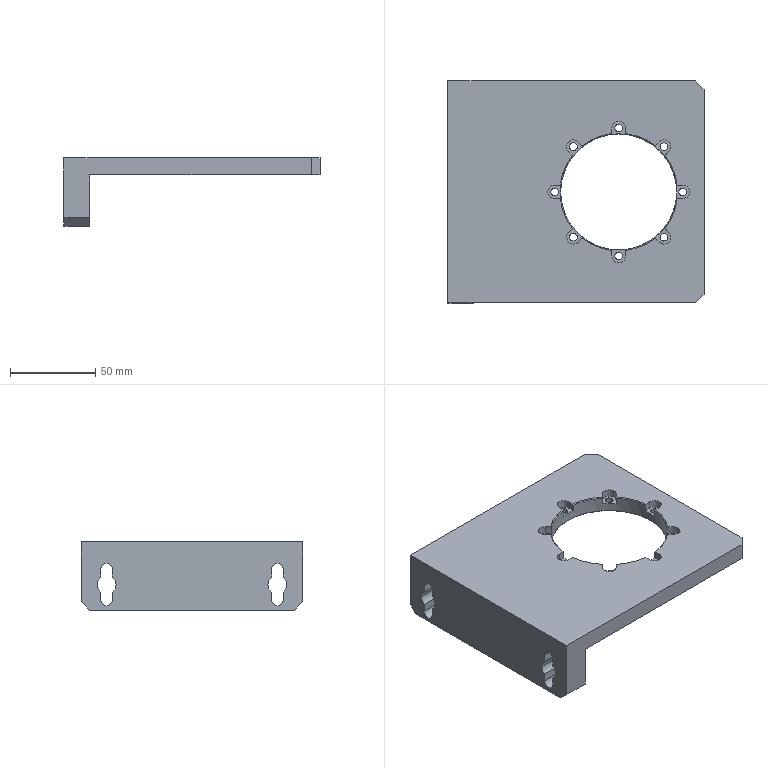NC program | NX | posted with a generic post | part box 150 x 130 x 40 mm
Lines 1 to 1320 of 2441:
N10 G17 G21 G94 G90
(FLOOR_WALL_COPY , TOOL : D80)
N12 T19 M6
N14 G54
N16 G17 G0 G90 X-123.5 Y68.497 B0. C0. S6500 M3
N18 G43 Z30. H19
N20 Z3.
N22 G94 G1 Z0. F1500.
N24 X-118.5
N26 X118.5
N28 Y15.999
N30 X-118.5
N32 Y-36.5
N34 X118.5
N36 X123.5
N38 Z3.
N40 G0 Z30.
N42 M5
(DRILLING_COPY_1 , TOOL : D6A45)
N44 T01 M6
N46 G54
N48 G17 G0 G90 X62.5 Y0. B0. C0. S5000 M3
N50 G43 Z30. H1
N52 G94 G81 G98 Z-1. F350. R3.
N54 X51.517 Y26.517
N56 X25. Y37.5
N58 X-1.517 Y26.517
N60 X-12.5 Y0.
N62 X-1.517 Y-26.517
N64 X25. Y-37.5
N66 X51.517 Y-26.517
N68 G80
N70 G0 X51.517 Y-26.517 Z30.
N72 M5
(DRILLING_COPY_COPY_COPY_2 , TOOL : 4.5ZT)
N74 T08 M6
N76 G54
N78 G17 G0 G90 X62.5 Y0. B0. C0. S2000 M3
N80 G43 Z30. H8
N82 G94 G83 G98 Z-12.852 F180. Q2. R3.
N84 X51.517 Y26.517
N86 X25. Y37.5
N88 X-1.517 Y26.517
N90 X-12.5 Y0.
N92 X-1.517 Y-26.517
N94 X25. Y-37.5
N96 X51.517 Y-26.517
N98 G80
N100 G0 X51.517 Y-26.517 Z30.
N102 M5
(ADAPTIVE_MILLING , TOOL : D10)
N104 T15 M6
N106 G54
N108 G17 G0 G90 X-90.269 Y-0.047 B0. C0. S9500 M3
N110 G43 Z30. H15
N112 Z-17.
N114 G94 G1 Z-20. F1000.
N116 X-87.817 Y-1.446 F3000.
N118 G3 X-83.547 Y-0.047 R3.035
N120 X-82.896 Y3.212 R9.612
N122 X-82.707 Y14.208 R174.736
N124 G1 X-82.705 Y22.408
N126 Y65.808
N128 X-82.703 Y65.908
N130 X-82.699 Y66.008
N132 X-82.694 Y66.108
N134 X-82.685 Y66.208
N136 G2 X-79.774 Y70.541 R6.036
N138 X-74.302 Y72.313 R13.071
N140 X-65.414 Y72.674 R78.607
N142 G1 X-63.814 Y72.681
N144 X-61.414 Y72.685
N146 X-56.914 Y72.687
N148 X75.786 Y72.688
N150 X75.886 Y72.687
N152 X75.986 Y72.683
N154 G2 X80.36 Y70.024 R5.852
N156 X82.27 Y64.605 R12.334
N158 X82.676 Y56.12 R67.698
N160 G1 X82.682 Y54.52
N162 X82.686 Y52.02
N164 X82.688 Y47.02
N166 X82.689 Y-0.98
N168 X82.696 Y-3.98
N170 X82.7 Y-6.98
N172 Y-9.98
N174 X82.696 Y-12.98
N176 X82.695 Y-13.78
N178 X82.696 Y-16.98
N180 X82.693 Y-20.08
N182 Y-20.68
N184 X82.696 Y-23.68
N186 X82.695 Y-26.68
N188 X82.693 Y-28.38
N190 X82.696 Y-31.38
N192 X82.695 Y-34.38
N194 X82.693 Y-35.98
N196 X82.696 Y-38.98
N198 X82.695 Y-41.98
N200 X82.693 Y-43.58
N202 X82.696 Y-46.58
N204 X82.695 Y-49.58
N206 X82.693 Y-51.18
N208 X82.696 Y-54.18
N210 G2 X82.665 Y-66.278 R754.805
N212 X79.782 Y-70.524 R6.056
N214 X74.315 Y-72.309 R12.987
N216 X66.028 Y-72.671 R72.365
N218 G1 X64.728 Y-72.677
N220 X62.828 Y-72.683
N222 X59.828 Y-72.686
N224 X52.328 Y-72.688
N226 X-75.772
N228 X-75.872 Y-72.687
N230 G2 X-80.233 Y-70.193 R5.761
N232 X-82.253 Y-64.714 R11.977
N234 X-82.677 Y-55.631 R69.388
N236 G1 X-82.683 Y-53.731
N238 X-82.687 Y-50.731
N240 X-82.688 Y-43.431
N242 Y-3.431
N244 X-82.686 Y-3.231
N246 X-82.684 Y-3.131
N248 G2 X-82.17 Y2.746 R196.765
N250 G3 X-81.919 Y14.44 R177.481
N252 G1 X-81.916 Y17.64
N254 X-81.914 Y25.44
N256 Y63.04
N258 X-81.913 Y63.14
N260 X-81.911 Y63.24
N262 X-81.902 Y63.44
N264 G2 X-78.052 Y69.525 R7.633
N266 X-71.898 Y71.461 R15.425
N268 X-62.412 Y71.864 R83.04
N270 G1 X-60.812 Y71.871
N272 X-58.412 Y71.875
N274 X-54.312 Y71.878
N276 X-36.512 Y71.879
N278 X73.088
N280 X73.188 Y71.878
N282 G2 X79.498 Y68.067 R7.587
N284 X81.456 Y61.921 R15.338
N286 X81.864 Y52.936 R76.536
N288 G1 X81.871 Y51.336
N290 X81.876 Y49.036
N292 X81.879 Y45.136
N294 X81.88 Y30.936
N296 Y1.736
N298 X81.889 Y-1.464
N300 X81.893 Y-4.564
N302 X81.894 Y-7.664
N304 X81.891 Y-10.764
N306 Y-11.064
N308 X81.894 Y-14.064
N310 X81.892 Y-17.064
N312 X81.89 Y-18.764
N314 X81.894 Y-21.964
N316 X81.893 Y-25.064
N318 X81.891 Y-26.964
N320 X81.894 Y-30.164
N322 Y-33.264
N324 X81.892 Y-35.564
N326 X81.894 Y-38.564
N328 X81.893 Y-41.564
N330 X81.892 Y-43.264
N332 X81.894 Y-46.264
N334 X81.893 Y-49.264
N336 X81.892 Y-50.864
N338 X81.894 Y-53.864
N340 G2 X81.859 Y-63.763 R364.257
N342 X77.841 Y-69.641 R7.736
N344 X71.558 Y-71.501 R16.073
N346 X61.469 Y-71.866 R97.349
N348 G1 X59.569 Y-71.872
N350 X56.769 Y-71.877
N352 X51.269 Y-71.879
N354 X-15.231 Y-71.88
N356 X-18.131 Y-71.887
N358 X-20.931 Y-71.89
N360 X-23.731 Y-71.889
N362 X-26.331 Y-71.885
N364 X-29.331 Y-71.887
N366 X-32.331 Y-71.884
N368 X-32.831
N370 X-35.831 Y-71.887
N372 X-38.831 Y-71.886
N374 X-40.431 Y-71.884
N376 X-43.431 Y-71.887
N378 X-46.431 Y-71.886
N380 X-48.031 Y-71.884
N382 X-51.031 Y-71.887
N384 X-54.031 Y-71.886
N386 X-55.631 Y-71.884
N388 X-58.631 Y-71.887
N390 X-61.631 Y-71.886
N392 X-63.231 Y-71.884
N394 X-66.231 Y-71.887
N396 G2 X-73.829 Y-71.845 R186.129
N398 X-79.625 Y-67.863 R7.744
N400 X-81.487 Y-61.683 R15.948
N402 X-81.863 Y-52.496 R84.129
N404 G1 X-81.87 Y-50.896
N406 X-81.875 Y-48.696
N408 X-81.878 Y-45.096
N410 X-81.88 Y-33.796
N412 X-81.879 Y-5.496
N414 X-81.876 Y-5.096
N416 G2 X-81.37 Y2.987 R183.688
N418 G3 X-81.126 Y17.983 R281.687
N420 G1 X-81.123 Y23.083
N422 X-81.122 Y60.383
N424 X-81.12 Y60.783
N426 X-81.113 Y61.083
N428 X-81.106 Y61.282
N430 G2 X-80.201 Y64.947 R9.916
N432 G3 X-79.936 Y66.425 R42.453
N434 G2 X-76.234 Y69.988 R5.268
N436 X-62.992 Y71.033 R77.349
N438 G1 X-61.792 Y71.045
N440 X-60.392 Y71.054
N442 X-58.392 Y71.062
N444 X-56.192 Y71.066
N446 X-52.192 Y71.069
N448 X-39.692 Y71.071
N450 X20.408
N452 X23.408 Y71.079
N454 X26.408 Y71.083
N456 X29.408
N458 X32.408 Y71.078
N460 X33.208 Y71.077
N462 X36.408 Y71.078
N464 X39.508 Y71.076
N466 X40.108 Y71.075
N468 X43.308 Y71.079
N470 X46.408 Y71.078
N472 X48.908 Y71.076
N474 X51.908 Y71.078
N476 X54.908 Y71.077
N478 X56.408 Y71.075
N480 X59.408 Y71.078
N482 X62.408 Y71.077
N484 X64.008 Y71.075
N486 X67.008 Y71.078
N488 G2 X72.006 Y71.008 R68.55
N490 X78.82 Y66.179 R8.85
N492 X80.698 Y59.378 R18.423
N494 X81.06 Y48.989 R104.039
N496 G1 X81.066 Y46.689
N498 X81.069 Y43.489
N500 X81.071 Y35.689
N502 Y4.389
N504 X81.081 Y1.089
N506 X81.087 Y-2.211
N508 X81.089 Y-5.511
N510 X81.087 Y-8.911
N512 X81.091 Y-12.111
N514 X81.092 Y-15.211
N516 X81.089 Y-18.311
N518 X81.093 Y-21.811
N520 X81.092 Y-24.911
N522 X81.09 Y-27.011
N524 X81.093 Y-30.211
N526 Y-33.311
N528 X81.091 Y-35.711
N530 X81.093 Y-38.711
N532 X81.092 Y-41.711
N534 X81.09 Y-43.311
N536 X81.094 Y-46.511
N538 X81.093 Y-49.611
N540 X81.091 Y-51.811
N542 X81.094 Y-54.811
N544 G2 X81.032 Y-61.909 R127.091
N546 X76.19 Y-68.822 R8.855
N548 X69.488 Y-70.683 R18.238
N550 X58.799 Y-71.06 R106.559
N552 G1 X56.499 Y-71.065
N554 X52.899 Y-71.069
N556 X44.199 Y-71.071
N558 X-12.501
N560 X-15.701 Y-71.08
N562 X-18.801 Y-71.084
N564 X-21.901 Y-71.085
N566 X-25.101 Y-71.082
N568 X-28.301 Y-71.086
N570 X-31.401
N572 X-33.901 Y-71.083
N574 X-36.901 Y-71.086
N576 X-39.901 Y-71.085
N578 X-41.501 Y-71.083
N580 X-44.501 Y-71.086
N582 X-47.501 Y-71.085
N584 X-49.101 Y-71.083
N586 X-52.301 Y-71.087
N588 X-55.401 Y-71.086
N590 X-57.901 Y-71.083
N592 X-60.901 Y-71.086
N594 X-63.901 Y-71.084
N596 X-65.101 Y-71.083
N598 X-68.101 Y-71.086
N600 G2 X-72.296 Y-70.977 R34.856
N602 X-74.971 Y-70.178 R12.895
N604 G1 X-75.067 Y-70.153
N606 X-75.165 Y-70.131
N608 X-75.187 Y-70.125
N610 X-76.234 Y-69.988
N612 X-76.331 Y-69.968
N614 X-76.425 Y-69.936
N616 G2 X-79.988 Y-66.234 R5.268
N618 X-81.039 Y-52.992 R78.181
N620 G1 X-81.049 Y-51.792
N622 X-81.057 Y-50.092
N624 X-81.064 Y-48.092
N626 X-81.068 Y-45.092
N628 X-81.071 Y-39.492
N630 Y-7.192
N632 G2 X-80.6 Y2.595 R173.692
N634 G3 X-80.335 Y19.791 R352.511
N636 G1 X-80.332 Y25.091
N638 X-80.331 Y57.691
N640 X-80.329 Y58.291
N642 X-80.324 Y58.791
N644 X-80.32 Y58.991
N646 X-80.315 Y59.191
N648 X-80.15 Y61.023
N650 G2 X-80.111 Y65.297 R63.737
N652 G1 X-79.968 Y66.331
N654 X-79.454 Y67.572
N656 X-78.637 Y68.637
N658 X-77.572 Y69.454
N660 X-76.331 Y69.968
N662 X-75.837 Y70.04
N664 X-75.099 Y70.137
N666 X-74.9 Y70.15
N668 G3 X-59.101 Y70.257 R879.606
N670 G1 X-56.601 Y70.266
N672 X-53.401 Y70.271
N674 X-52.601 Y70.272
N676 X-49.601 Y70.271
N678 X-46.601 Y70.274
N680 X-43.601 Y70.272
N682 X-40.601 Y70.273
N684 X-39.101 Y70.274
N686 X-36.101 Y70.272
N688 X-33.101 Y70.273
N690 X-31.501 Y70.274
N692 X-28.501 Y70.272
N694 X-25.501 Y70.273
N696 X-24.001 Y70.275
N698 X-21.001 Y70.272
N700 X-18.001 Y70.273
N702 X-16.401 Y70.275
N704 X-13.401 Y70.272
N706 X-10.401 Y70.273
N708 X-8.801 Y70.275
N710 X-5.801 Y70.272
N712 X-2.801 Y70.273
N714 X-1.301 Y70.275
N716 X1.699 Y70.272
N718 X4.699 Y70.273
N720 X6.299 Y70.275
N722 X9.299 Y70.272
N724 X12.299 Y70.273
N726 X13.899 Y70.274
N728 X16.899 Y70.272
N730 X19.899 Y70.273
N732 X22.899 Y70.278
N734 X24.899 Y70.283
N736 X27.899 Y70.285
N738 X28.499
N740 X31.499 Y70.282
N742 X34.499
N744 X35.399 Y70.283
N746 X38.399 Y70.278
N748 X41.399
N750 X44.399 Y70.281
N752 X47.399 Y70.279
N754 X50.399 Y70.28
N756 X51.599 Y70.282
N758 X54.599 Y70.279
N760 X57.599 Y70.28
N762 X59.199 Y70.281
N764 X62.199 Y70.279
N766 G2 X70.097 Y70.216 R155.086
N768 X77.918 Y64.879 R9.64
N770 G3 X79.399 Y62.654 R9.765
N772 G2 X80.15 Y59.9 R5.821
N774 G3 X80.255 Y49.201 R795.028
N776 G1 X80.265 Y46.901
N778 X80.271 Y43.701
N780 X80.272 Y43.401
N782 Y40.401
N784 X80.275 Y37.901
N786 X80.272 Y34.901
N788 X80.273 Y31.901
N790 X80.275 Y30.601
N792 X80.272 Y27.601
N794 X80.273 Y24.601
N796 X80.275 Y23.001
N798 X80.272 Y20.001
N800 X80.273 Y17.001
N802 X80.275 Y15.401
N804 X80.272 Y12.401
N806 X80.273 Y9.401
N808 X80.275 Y7.801
N810 X80.272 Y4.801
N812 Y3.801
N814 X80.281 Y0.601
N816 X80.286 Y-2.499
N818 X80.287 Y-5.599
N820 X80.285 Y-8.299
N822 X80.29 Y-11.499
N824 Y-14.599
N826 X80.288 Y-17.699
N828 X80.291 Y-20.899
N830 Y-23.999
N832 X80.289 Y-26.299
N834 X80.292 Y-29.499
N836 Y-32.599
N838 X80.289 Y-35.099
N840 X80.292 Y-38.099
N842 X80.291 Y-41.099
N844 X80.289 Y-42.599
N846 G2 X80.258 Y-59.698 R947.533
N848 X74.891 Y-67.919 R9.657
N850 G3 X72.654 Y-69.399 R9.648
N852 G2 X69.9 Y-70.15 R5.821
N854 G3 X59.301 Y-70.254 R763.229
N856 G1 X57.101 Y-70.263
N858 X53.901 Y-70.27
N860 X50.601 Y-70.271
N862 X48.501 Y-70.274
N864 X45.501 Y-70.272
N866 X42.501 Y-70.273
N868 X41.301 Y-70.274
N870 X38.301 Y-70.272
N872 X35.301 Y-70.273
N874 X33.701 Y-70.274
N876 X30.701 Y-70.272
N878 X27.701 Y-70.273
N880 X26.201 Y-70.274
N882 X23.201 Y-70.272
N884 X20.201 Y-70.273
N886 X18.601 Y-70.275
N888 X15.601 Y-70.272
N890 X12.601 Y-70.273
N892 X11.001 Y-70.275
N894 X8.001 Y-70.272
N896 X5.001 Y-70.273
N898 X3.501 Y-70.274
N900 X0.501 Y-70.272
N902 X-2.499 Y-70.273
N904 X-4.099 Y-70.275
N906 X-7.099 Y-70.272
N908 X-10.099 Y-70.273
N910 X-13.099 Y-70.278
N912 X-15.099 Y-70.283
N914 X-18.099 Y-70.285
N916 X-20.099 Y-70.288
N918 X-23.099 Y-70.286
N920 X-26.099 Y-70.288
N922 X-27.399 Y-70.29
N924 X-30.399 Y-70.288
N926 X-33.399 Y-70.289
N928 X-34.299 Y-70.29
N930 X-37.299 Y-70.287
N932 X-40.299 Y-70.288
N934 X-42.099 Y-70.29
N936 X-45.099 Y-70.287
N938 X-48.099 Y-70.288
N940 X-49.799 Y-70.29
N942 X-52.799 Y-70.288
N944 X-55.799 Y-70.289
N946 X-56.499
N948 X-59.399 Y-70.286
N950 G2 X-69.798 Y-70.245 R420.97
N952 G1 X-69.997 Y-70.231
N954 X-70.197 Y-70.213
N956 X-70.396 Y-70.192
N958 X-70.594 Y-70.168
N960 X-70.694 Y-70.158
N962 X-70.793 Y-70.15
N964 X-74.9
N966 X-75.099 Y-70.137
N968 X-75.198 Y-70.124
N970 G3 X-76.434 Y-70.217 R3.145
N972 G1 X-81.889 Y-71.791
N974 G2 X-85.759 Y-68.817 R3.033
N976 G1 Z-17.
N978 G0 Z30.
N980 X-82.829 Y73.315
N982 Z-17.
N984 G1 Z-20. F1000.
N986 G2 X-78.303 Y75.887 R3.033 F3000.
N988 G1 X-68.896 Y70.545
N990 G3 X-67.4 Y70.15 R3.105
N992 G1 X69.9
N994 X70.099 Y70.137
N996 G2 X73.562 Y68.702 R5.4
N998 G1 X73.712 Y68.571
N1000 X78.571 Y63.712
N1002 X79.022 Y63.15
N1004 X79.454 Y62.572
N1006 X79.968 Y61.331
N1008 X80.071 Y60.617
N1010 X80.15 Y59.9
N1012 Y-59.9
N1014 X80.137 Y-60.099
N1016 G2 X78.702 Y-63.562 R5.4
N1018 G1 X78.571 Y-63.712
N1020 X73.712 Y-68.571
N1022 X73.15 Y-69.022
N1024 X72.572 Y-69.454
N1026 X71.331 Y-69.968
N1028 X70.617 Y-70.071
N1030 X69.9 Y-70.15
N1032 X-74.9
N1034 X-75.617 Y-70.071
N1036 X-76.331 Y-69.968
N1038 X-77.572 Y-69.454
N1040 X-78.637 Y-68.637
N1042 X-79.454 Y-67.572
N1044 X-79.968 Y-66.331
N1046 X-80.053 Y-65.738
N1048 X-80.137 Y-65.099
N1050 X-80.15 Y-64.9
N1052 G3 X-80.254 Y-50.001 R826.107
N1054 G1 X-80.264 Y-47.601
N1056 X-80.271 Y-44.401
N1058 Y-44.001
N1060 X-80.272 Y-41.001
N1062 X-80.274 Y-38.501
N1064 X-80.272 Y-35.501
N1066 X-80.274 Y-32.501
N1068 X-80.275 Y-31.301
N1070 X-80.272 Y-28.301
N1072 X-80.273 Y-25.301
N1074 X-80.275 Y-23.701
N1076 X-80.272 Y-20.701
N1078 X-80.273 Y-17.701
N1080 X-80.275 Y-16.101
N1082 X-80.272 Y-13.101
N1084 G2 X-80.15 Y-3.703 R204.302
N1086 G1 Y61.097
N1088 G3 X-81.032 Y63.343 R3.335
N1090 X-83.137 Y64.382 Z-19.9 R3.335
N1092 X-86.75 Y61.097 R3.305
N1094 G1 Y-57.6
N1096 G3 X-82.982 Y-60.867 R3.305
N1098 X-80.928 Y-59.729 Z-20. R3.335
N1100 X-80.15 Y-57.6 R3.336
N1102 G1 Y-3.7
N1104 G3 X-83.078 Y-0.672 R3.036
N1106 G1 X-86.343 Y-0.562
N1108 Z-17.
N1110 G0 Z30.
N1112 X-90.271 Y-0.049
N1114 Z-37.
N1116 G1 Z-40. F1000.
N1118 X-87.819 Y-1.448 F3000.
N1120 G3 X-83.549 Y-0.049 R3.035
N1122 X-82.898 Y3.21 R9.612
N1124 X-82.709 Y14.207 R174.736
N1126 G1 X-82.707 Y22.407
N1128 Y65.807
N1130 X-82.705 Y65.907
N1132 X-82.701 Y66.007
N1134 X-82.695 Y66.106
N1136 X-82.687 Y66.206
N1138 G2 X-79.778 Y70.541 R6.037
N1140 X-74.307 Y72.314 R13.032
N1142 X-65.419 Y72.676 R78.45
N1144 G1 X-63.919 Y72.682
N1146 X-61.619 Y72.687
N1148 X-57.419 Y72.689
N1150 X-27.519 Y72.69
N1152 X75.781
N1154 X75.881 Y72.689
N1156 G2 X80.24 Y70.191 R5.757
N1158 X82.27 Y64.611 R12.073
N1160 X82.667 Y56.727 R62.897
N1162 G1 X82.676 Y55.527
N1164 X82.682 Y53.927
N1166 X82.687 Y51.627
N1168 X82.689 Y47.527
N1170 X82.69 Y14.427
N1172 X82.691 Y-7.273
N1174 X82.698 Y-10.273
N1176 X82.702 Y-13.273
N1178 Y-16.273
N1180 X82.698 Y-19.273
N1182 X82.697 Y-20.073
N1184 X82.698 Y-23.273
N1186 X82.695 Y-26.373
N1188 Y-26.973
N1190 X82.698 Y-29.973
N1192 X82.697 Y-32.973
N1194 X82.695 Y-34.673
N1196 X82.698 Y-37.673
N1198 X82.697 Y-40.673
N1200 X82.695 Y-42.273
N1202 X82.698 Y-45.273
N1204 X82.697 Y-48.273
N1206 X82.695 Y-49.873
N1208 X82.698 Y-52.873
N1210 X82.697 Y-55.873
N1212 X82.695 Y-57.473
N1214 X82.698 Y-60.473
N1216 G2 X82.658 Y-66.371 R131.179
N1218 X79.624 Y-70.628 R6.152
N1220 X74.129 Y-72.335 R13.448
N1222 X65.04 Y-72.682 R83.457
N1224 G1 X62.74 Y-72.687
N1226 X58.44 Y-72.689
N1228 X8.74 Y-72.69
N1230 X-75.86 Y-72.689
N1232 X-75.96 Y-72.686
N1234 X-76.06 Y-72.681
N1236 G2 X-80.459 Y-69.881 R5.939
N1238 X-82.295 Y-64.433 R12.732
N1240 X-82.678 Y-55.147 R77.923
N1242 G1 X-82.684 Y-53.447
N1244 X-82.688 Y-50.847
N1246 X-82.69 Y-45.447
N1248 Y-3.347
N1250 X-82.686 Y-3.147
N1252 X-82.681 Y-2.947
N1254 G2 X-82.147 Y3.129 R700.412
N1256 G3 X-81.918 Y17.225 R247.329
N1258 G1 X-81.916 Y23.825
N1260 Y63.025
N1262 X-81.915 Y63.125
N1264 X-81.913 Y63.225
N1266 X-81.905 Y63.425
N1268 X-81.892 Y63.624
N1270 G2 X-77.984 Y69.571 R7.687
N1272 X-71.719 Y71.486 R15.754
N1274 X-61.732 Y71.868 R93.067
N1276 G1 X-59.932 Y71.874
N1278 X-57.432 Y71.878
N1280 X-52.632 Y71.881
N1282 X60.968
N1284 X73.068
N1286 X73.168 Y71.88
N1288 G2 X79.489 Y68.087 R7.588
N1290 X81.478 Y61.745 R15.429
N1292 X81.864 Y52.358 R85.367
N1294 G1 X81.871 Y50.858
N1296 X81.876 Y48.758
N1298 X81.88 Y45.458
N1300 X81.881 Y37.358
N1302 X81.882 Y-4.542
N1304 X81.891 Y-7.742
N1306 X81.895 Y-10.842
N1308 X81.896 Y-13.942
N1310 X81.893 Y-17.042
N1312 Y-17.342
N1314 X81.896 Y-20.342
N1316 X81.894 Y-23.342
N1318 X81.892 Y-25.042
N1320 X81.895 Y-28.242
N1322 X81.894 Y-31.342
N1324 X81.893 Y-33.242
N1326 X81.896 Y-36.442
N1328 Y-39.542
N1330 X81.893 Y-41.842
N1332 X81.896 Y-44.842
N1334 X81.895 Y-47.842
N1336 X81.893 Y-49.542
N1338 X81.896 Y-52.542
N1340 X81.895 Y-55.542
N1342 X81.893 Y-57.142
N1344 X81.896 Y-60.142
N1346 G2 X81.815 Y-64.138 R36.087
N1348 X77.602 Y-69.779 R7.882
N1350 X71.185 Y-71.546 R17.008
N1352 X61.695 Y-71.868 R100.448
N1354 G1 X59.895 Y-71.875
N1356 X57.295 Y-71.879
N1358 X52.095 Y-71.881
N1360 X-73.105
N1362 X-73.205 Y-71.879
N1364 X-73.405 Y-71.873
N1366 G2 X-79.508 Y-68.052 R7.626
N1368 X-81.459 Y-61.904 R15.357
N1370 X-81.862 Y-52.618 R81.436
N1372 G1 X-81.87 Y-51.218
N1374 X-81.875 Y-49.418
N1376 X-81.879 Y-46.618
N1378 X-81.881 Y-40.818
N1380 Y-5.518
N1382 X-81.88 Y-5.318
N1384 G2 X-81.389 Y2.765 R158.22
N1386 G3 X-81.129 Y17.161 R254.609
N1388 G1 X-81.126 Y21.361
N1390 X-81.125 Y34.261
N1392 X-81.124 Y60.361
N1394 X-81.122 Y60.761
N1396 X-81.116 Y61.06
N1398 X-81.108 Y61.26
N1400 G2 X-80.18 Y65.021 R10.687
N1402 G1 X-80.154 Y65.118
N1404 X-80.13 Y65.215
N1406 X-80.109 Y65.313
N1408 X-79.988 Y66.234
N1410 X-79.968 Y66.331
N1412 X-79.936 Y66.425
N1414 G2 X-76.234 Y69.988 R5.268
N1416 X-62.892 Y71.035 R77.561
N1418 G1 X-61.692 Y71.046
N1420 X-60.292 Y71.055
N1422 X-58.392 Y71.063
N1424 X-56.192 Y71.068
N1426 X-52.392 Y71.071
N1428 X-42.192 Y71.072
N1430 X-2.992 Y71.073
N1432 X0.008 Y71.081
N1434 X3.008 Y71.085
N1436 X6.008 Y71.084
N1438 X9.008 Y71.08
N1440 X9.808 Y71.079
N1442 X13.008 Y71.08
N1444 X16.108 Y71.078
N1446 X16.708 Y71.077
N1448 X19.908 Y71.081
N1450 X23.008 Y71.08
N1452 X25.508 Y71.077
N1454 X28.708 Y71.081
N1456 X31.808 Y71.08
N1458 X34.008 Y71.077
N1460 X37.008 Y71.08
N1462 X40.008 Y71.079
N1464 X41.408 Y71.077
N1466 X44.408 Y71.08
N1468 X47.408 Y71.079
N1470 X49.008 Y71.077
N1472 X52.008 Y71.08
N1474 X55.008 Y71.079
N1476 X56.608 Y71.077
N1478 X59.808 Y71.081
N1480 G2 X71.707 Y71.039 R440.492
N1482 X78.724 Y66.358 R8.791
N1484 X80.684 Y59.481 R17.918
N1486 X81.06 Y48.492 R113.184
N1488 G1 X81.066 Y46.392
N1490 X81.07 Y43.492
N1492 X81.073 Y37.592
N1494 Y-1.808
N1496 X81.082 Y-5.008
N1498 X81.087 Y-8.108
N1500 X81.088 Y-11.908
N1502 X81.087 Y-15.908
N1504 X81.095 Y-19.108
N1506 X81.098 Y-22.208
N1508 Y-25.308
N1510 X81.093 Y-28.408
N1512 X81.092 Y-29.408
N1514 X81.093 Y-32.408
N1516 X81.091 Y-34.508
N1518 X81.096 Y-37.508
N1520 Y-40.508
N1522 X81.093 Y-43.408
N1524 X81.096 Y-46.608
N1526 X81.095 Y-49.708
N1528 X81.092 Y-51.908
N1530 X81.095 Y-54.908
N1532 X81.094 Y-57.908
N1534 X81.092 Y-59.108
N1536 G2 X80.835 Y-63.088 R16.768
N1538 X75.843 Y-69.006 R9.072
N1540 X68.999 Y-70.74 R19.471
N1542 X58.107 Y-71.062 R129.678
N1544 G1 X55.907 Y-71.067
N1546 X52.507 Y-71.071
N1548 X44.007 Y-71.072
N1550 X-70.693
N1552 X-70.993 Y-71.069
N1554 X-71.093 Y-71.066
N1556 G2 X-74.868 Y-70.203 R9.973
N1558 G1 X-74.964 Y-70.176
N1560 X-75.061 Y-70.152
N1562 X-75.168 Y-70.128
N1564 X-76.234 Y-69.988
N1566 X-76.331 Y-69.968
N1568 X-76.425 Y-69.936
N1570 G2 X-79.988 Y-66.234 R5.268
N1572 X-81.049 Y-52.292 R81.817
N1574 G1 X-81.057 Y-50.792
N1576 X-81.065 Y-48.592
N1578 X-81.069 Y-45.792
N1580 X-81.072 Y-40.892
N1582 X-81.073 Y-11.392
N1584 X-81.072 Y-7.092
N1586 G2 X-80.606 Y2.595 R173.405
N1588 G3 X-80.337 Y19.091 R338.312
N1590 G1 X-80.334 Y23.591
N1592 X-80.333 Y37.691
N1594 Y57.591
N1596 X-80.33 Y58.391
N1598 X-80.326 Y58.791
N1600 X-80.319 Y59.091
N1602 G2 X-80.15 Y61.082 R56.218
N1604 G1 Y64.9
N1606 X-80.137 Y65.099
N1608 X-80.098 Y65.396
N1610 X-79.968 Y66.331
N1612 X-79.454 Y67.572
N1614 X-78.637 Y68.637
N1616 X-77.572 Y69.454
N1618 X-76.331 Y69.968
N1620 X-75.837 Y70.04
N1622 X-75.099 Y70.137
N1624 X-74.9 Y70.15
N1626 G3 X-59.001 Y70.258 R888.706
N1628 G1 X-56.501 Y70.267
N1630 X-53.501 Y70.272
N1632 X-52.901 Y70.273
N1634 X-49.901
N1636 X-47.101 Y70.276
N1638 X-44.101 Y70.274
N1640 X-41.101 Y70.275
N1642 X-39.801 Y70.276
N1644 X-36.801 Y70.274
N1646 X-33.801 Y70.275
N1648 X-32.201 Y70.276
N1650 X-29.201 Y70.274
N1652 X-26.201 Y70.275
N1654 X-24.601 Y70.276
N1656 X-21.601 Y70.274
N1658 X-18.601 Y70.275
N1660 X-17.101 Y70.276
N1662 X-14.101 Y70.273
N1664 X-11.101 Y70.275
N1666 X-9.501 Y70.276
N1668 X-6.501 Y70.274
N1670 X-3.501 Y70.275
N1672 X-0.501 Y70.28
N1674 X1.499 Y70.285
N1676 X4.699 Y70.286
N1678 X5.499 Y70.287
N1680 X8.699 Y70.282
N1682 X11.799
N1684 X13.699 Y70.283
N1686 X16.699 Y70.278
N1688 X19.699
N1690 X22.699 Y70.281
N1692 X25.699 Y70.278
N1694 X28.699 Y70.28
N1696 X30.399 Y70.282
N1698 X33.399 Y70.28
N1700 X36.399 Y70.281
N1702 X37.599 Y70.283
N1704 X40.599 Y70.28
N1706 X43.599 Y70.281
N1708 X45.199 Y70.282
N1710 X48.199 Y70.28
N1712 X51.199 Y70.281
N1714 X52.699 Y70.282
N1716 X55.699 Y70.28
N1718 X58.699 Y70.281
N1720 X60.699 Y70.283
N1722 X63.899 Y70.28
N1724 G2 X70.197 Y70.208 R96.937
N1726 X77.965 Y64.794 R9.65
N1728 G3 X79.399 Y62.654 R9.527
N1730 G2 X80.15 Y59.9 R5.821
N1732 G3 X80.257 Y48.301 R824.167
N1734 G1 X80.267 Y46.001
N1736 X80.273 Y42.801
N1738 Y42.301
N1740 X80.274 Y39.301
N1742 X80.276 Y36.801
N1744 X80.274 Y33.801
N1746 X80.275 Y30.801
N1748 X80.277 Y29.501
N1750 X80.274 Y26.501
N1752 X80.275 Y23.501
N1754 X80.277 Y21.901
N1756 X80.274 Y18.901
N1758 X80.275 Y15.901
N1760 X80.277 Y14.301
N1762 X80.274 Y11.301
N1764 X80.275 Y8.301
N1766 X80.277 Y6.801
N1768 X80.274 Y3.801
N1770 X80.275 Y0.801
N1772 X80.28 Y-2.199
N1774 X80.285 Y-4.199
N1776 X80.287 Y-7.199
N1778 X80.29 Y-9.399
N1780 X80.289 Y-12.399
N1782 X80.291 Y-15.399
N1784 X80.298 Y-18.399
N1786 Y-18.699
N1788 X80.299 Y-21.699
N1790 X80.301 Y-23.499
N1792 X80.298 Y-26.499
N1794 X80.299 Y-29.299
N1796 X80.294 Y-32.199
N1798 X80.293 Y-34.999
N1800 X80.297 Y-37.799
N1802 X80.298 Y-38.699
N1804 X80.297 Y-41.699
N1806 X80.299 Y-44.699
N1808 X80.3 Y-45.399
N1810 X80.297 Y-48.399
N1812 X80.298 Y-51.399
N1814 X80.299 Y-52.499
N1816 X80.296 Y-55.499
N1818 Y-58.199
N1820 X80.295 Y-58.499
N1822 X80.291 Y-58.899
N1824 X80.284 Y-59.199
N1826 X80.272 Y-59.499
N1828 G2 X74.897 Y-67.92 R9.669
N1830 G3 X72.654 Y-69.399 R9.583
N1832 G2 X69.9 Y-70.15 R5.821
N1834 G3 X58.501 Y-70.257 R812.566
N1836 G1 X56.101 Y-70.266
N1838 X53.101 Y-70.272
N1840 X52.701 Y-70.273
N1842 X49.701
N1844 X47.301 Y-70.276
N1846 X44.301 Y-70.273
N1848 X41.301 Y-70.275
N1850 X39.901 Y-70.276
N1852 X36.901 Y-70.274
N1854 X33.901 Y-70.275
N1856 X32.301 Y-70.276
N1858 X29.301 Y-70.274
N1860 X26.301 Y-70.275
N1862 X24.701 Y-70.276
N1864 X21.701 Y-70.273
N1866 X18.701 Y-70.275
N1868 X17.101 Y-70.276
N1870 X14.101 Y-70.274
N1872 X11.101 Y-70.275
N1874 X9.501 Y-70.276
N1876 X6.501 Y-70.274
N1878 X3.501 Y-70.275
N1880 X2.001 Y-70.276
N1882 X-0.999 Y-70.273
N1884 X-3.999 Y-70.275
N1886 X-5.599 Y-70.276
N1888 X-8.599 Y-70.274
N1890 X-11.599 Y-70.275
N1892 X-13.099 Y-70.276
N1894 X-16.099 Y-70.274
N1896 X-19.099 Y-70.275
N1898 X-20.699 Y-70.276
N1900 X-23.699 Y-70.274
N1902 X-26.699 Y-70.275
N1904 X-28.299 Y-70.276
N1906 X-31.299 Y-70.274
N1908 X-34.299 Y-70.275
N1910 X-35.999 Y-70.276
N1912 X-38.999 Y-70.274
N1914 X-41.999 Y-70.275
N1916 X-43.599 Y-70.276
N1918 X-46.599 Y-70.274
N1920 X-49.599 Y-70.275
N1922 X-51.199 Y-70.276
N1924 X-54.199 Y-70.274
N1926 G2 X-69.698 Y-70.241 R869.795
N1928 G1 X-69.898 Y-70.228
N1930 X-70.097 Y-70.212
N1932 X-70.296 Y-70.192
N1934 X-70.495 Y-70.17
N1936 X-70.594 Y-70.159
N1938 X-70.699 Y-70.15
N1940 X-74.9
N1942 X-75.099 Y-70.137
N1944 X-75.198 Y-70.124
N1946 G3 X-76.434 Y-70.217 R3.145
N1948 G1 X-81.889 Y-71.791
N1950 G2 X-85.759 Y-68.817 R3.033
N1952 G1 Z-37.
N1954 G0 Z30.
N1956 X-82.829 Y73.315
N1958 Z-37.
N1960 G1 Z-40. F1000.
N1962 G2 X-78.303 Y75.887 R3.033 F3000.
N1964 G1 X-68.896 Y70.545
N1966 G3 X-67.4 Y70.15 R3.105
N1968 G1 X69.9
N1970 X70.099 Y70.137
N1972 G2 X73.562 Y68.702 R5.4
N1974 G1 X73.712 Y68.571
N1976 X78.571 Y63.712
N1978 X79.022 Y63.15
N1980 X79.454 Y62.572
N1982 X79.968 Y61.331
N1984 X80.071 Y60.617
N1986 X80.15 Y59.9
N1988 Y-59.9
N1990 X80.137 Y-60.099
N1992 G2 X78.702 Y-63.562 R5.4
N1994 G1 X78.571 Y-63.712
N1996 X73.712 Y-68.571
N1998 X73.15 Y-69.022
N2000 X72.572 Y-69.454
N2002 X71.331 Y-69.968
N2004 X70.617 Y-70.071
N2006 X69.9 Y-70.15
N2008 X-74.9
N2010 X-75.617 Y-70.071
N2012 X-76.331 Y-69.968
N2014 X-77.572 Y-69.454
N2016 X-78.637 Y-68.637
N2018 X-79.454 Y-67.572
N2020 X-79.968 Y-66.331
N2022 X-80.053 Y-65.738
N2024 X-80.137 Y-65.099
N2026 X-80.15 Y-64.9
N2028 G3 X-80.257 Y-49.901 R842.567
N2030 G1 X-80.267 Y-47.501
N2032 X-80.272 Y-44.501
N2034 X-80.273 Y-44.001
N2036 Y-41.001
N2038 X-80.276 Y-38.501
N2040 X-80.274 Y-35.501
N2042 X-80.275 Y-32.501
N2044 X-80.277 Y-31.201
N2046 X-80.274 Y-28.201
N2048 X-80.275 Y-25.201
N2050 X-80.277 Y-23.701
N2052 X-80.274 Y-20.701
N2054 X-80.275 Y-17.701
N2056 X-80.277 Y-16.201
N2058 X-80.274 Y-13.201
N2060 G2 X-80.15 Y-3.603 R210.032
N2062 G1 Y61.097
N2064 G3 X-81.032 Y63.343 R3.335
N2066 X-83.137 Y64.382 Z-39.9 R3.335
N2068 X-86.75 Y61.097 R3.305
N2070 G1 Y-57.6
N2072 G3 X-82.982 Y-60.867 R3.305
N2074 X-80.928 Y-59.729 Z-40. R3.335
N2076 X-80.15 Y-57.6 R3.336
N2078 G1 Y-3.6
N2080 G3 X-83.078 Y-0.572 R3.036
N2082 G1 X-86.344 Y-0.462
N2084 Z-37.
N2086 G0 Z30.
(ADAPTIVE_MILLING_COPY , TOOL : D10)
N2088 X23.369 Y4.134
N2090 Z3.
N2092 G3 X23.369 Y4.134 Z2.753 I1.77 J-4.137 F1000.
N2094 X23.369 Y4.134 Z2.507 I1.77 J-4.137
N2096 X23.369 Y4.134 Z2.26 I1.77 J-4.137
N2098 X23.369 Y4.134 Z2.013 I1.77 J-4.137
N2100 X23.369 Y4.134 Z1.766 I1.77 J-4.137
N2102 X23.369 Y4.134 Z1.52 I1.77 J-4.137
N2104 X23.369 Y4.134 Z1.273 I1.77 J-4.137
N2106 X23.369 Y4.134 Z1.026 I1.77 J-4.137
N2108 X23.369 Y4.134 Z0.779 I1.77 J-4.137
N2110 X23.369 Y4.134 Z0.533 I1.77 J-4.137
N2112 X23.369 Y4.134 Z0.286 I1.77 J-4.137
N2114 X23.369 Y4.134 Z0.039 I1.77 J-4.137
N2116 X23.369 Y4.134 Z-0.208 I1.77 J-4.137
N2118 X23.369 Y4.134 Z-0.454 I1.77 J-4.137
N2120 X23.369 Y4.134 Z-0.701 I1.77 J-4.137
N2122 X23.369 Y4.134 Z-0.948 I1.77 J-4.137
N2124 X23.369 Y4.134 Z-1.195 I1.77 J-4.137
N2126 X23.369 Y4.134 Z-1.441 I1.77 J-4.137
N2128 X23.369 Y4.134 Z-1.688 I1.77 J-4.137
N2130 X23.369 Y4.134 Z-1.935 I1.77 J-4.137
N2132 X23.369 Y4.134 Z-2.182 I1.77 J-4.137
N2134 X23.369 Y4.134 Z-2.428 I1.77 J-4.137
N2136 X23.369 Y4.134 Z-2.675 I1.77 J-4.137
N2138 X23.369 Y4.134 Z-2.922 I1.77 J-4.137
N2140 X23.369 Y4.134 Z-3.169 I1.77 J-4.137
N2142 X23.369 Y4.134 Z-3.415 I1.77 J-4.137
N2144 X23.369 Y4.134 Z-3.662 I1.77 J-4.137
N2146 X23.369 Y4.134 Z-3.909 I1.77 J-4.137
N2148 X23.369 Y4.134 Z-4.156 I1.77 J-4.137
N2150 X23.369 Y4.134 Z-4.402 I1.77 J-4.137
N2152 X23.369 Y4.134 Z-4.649 I1.77 J-4.137
N2154 X23.369 Y4.134 Z-4.896 I1.77 J-4.137
N2156 X23.369 Y4.134 Z-5.143 I1.77 J-4.137
N2158 X23.369 Y4.134 Z-5.389 I1.77 J-4.137
N2160 X23.369 Y4.134 Z-5.636 I1.77 J-4.137
N2162 X23.369 Y4.134 Z-5.883 I1.77 J-4.137
N2164 X23.369 Y4.134 Z-6.13 I1.77 J-4.137
N2166 X23.369 Y4.134 Z-6.376 I1.77 J-4.137
N2168 X23.369 Y4.134 Z-6.623 I1.77 J-4.137
N2170 X23.369 Y4.134 Z-6.87 I1.77 J-4.137
N2172 X23.369 Y4.134 Z-7.117 I1.77 J-4.137
N2174 X23.369 Y4.134 Z-7.363 I1.77 J-4.137
N2176 X23.369 Y4.134 Z-7.61 I1.77 J-4.137
N2178 X23.369 Y4.134 Z-7.857 I1.77 J-4.137
N2180 X23.369 Y4.134 Z-8.104 I1.77 J-4.137
N2182 X23.369 Y4.134 Z-8.35 I1.77 J-4.137
N2184 X23.369 Y4.134 Z-8.597 I1.77 J-4.137
N2186 X23.369 Y4.134 Z-8.844 I1.77 J-4.137
N2188 X23.369 Y4.134 Z-9.091 I1.77 J-4.137
N2190 X23.369 Y4.134 Z-9.337 I1.77 J-4.137
N2192 X23.369 Y4.134 Z-9.584 I1.77 J-4.137
N2194 X23.369 Y4.134 Z-9.831 I1.77 J-4.137
N2196 X29.639 Y-0.004 Z-10. R-4.5
N2198 X28.98 Y-2.357 R-4.5 F3000.
N2200 X23.481 Y4.572 R4.637
N2202 X29.226 Y-2.692 R-4.873
N2204 X22.467 Y4.507 R5.039
N2206 X29.314 Y-3.229 R-5.255
N2208 X21.935 Y4.641 R5.444
N2210 X29.426 Y-3.722 R-5.655
N2212 X21.603 Y4.903 R5.851
N2214 X29.817 Y-3.908 R-6.067
N2216 X20.909 Y4.888 R6.273
N2218 X30.04 Y-4.301 R-6.49
N2220 X20.972 Y5.502 R6.703
N2222 X30.071 Y-4.908 R-6.927
N2224 X20.676 Y5.838 R7.148
N2226 X30.428 Y-5.19 R-7.377
N2228 X20.285 Y6.115 R7.604
N2230 X30.878 Y-5.399 R-7.841
N2232 X19.788 Y6.319 R8.076
N2234 X30.846 Y-6.094 R-8.314
N2236 X19.824 Y6.966 R8.552
N2238 X18.216 Y-5.368 R8.795
N2240 X30.557 Y-6.97 R8.795
N2242 X19.426 Y7.275 R-9.039
N2244 X31.021 Y-7.236 R-9.287
N2246 X19.24 Y7.76 R9.535
N2248 X30.561 Y-8.19 R9.786
N2250 X19.657 Y8.667 R10.038
N2252 X30.957 Y-8.546 R-10.296
N2254 X33.825 Y6.104 R10.556
N2256 X19.179 Y8.974 R10.556
N2258 X16.184 Y-6.025 R10.816
N2260 X31.139 Y-9.05 R10.816
N2262 X19.723 Y9.916 R11.076
N2264 X15.236 Y-5.484 R11.343
N2266 X30.69 Y-9.942 R11.343
N2268 X19.266 Y10.276 R-11.611
N2270 X31.254 Y-10.239 R-11.881
N2272 X19.896 Y11.211 R12.149
N2274 X30.753 Y-11.13 R-12.421
N2276 X19.873 Y11.803 R12.694
N2278 X13.331 Y-5.333 R12.97
N2280 X30.451 Y-11.882 R12.97
N2282 X20.55 Y12.675 R13.246
N2284 X29.914 Y-12.699 R-13.523
N2286 X21.492 Y13.555 R13.801
N2288 X28.623 Y-13.692 R14.083
N2290 X22.702 Y14.399 R14.366
N2292 X10.703 Y-2.491 R14.65
N2294 X27.575 Y-14.493 R14.65
N2296 X25.826 Y15.148 R14.931
N2298 X24.079 Y-15.228 R15.214
N2300 X29.205 Y15.186 R15.497
N2302 X20.348 Y-15.09 R15.776
N2304 X35.486 Y12.519 R16.051
N2306 X10.751 Y-7.88 R16.309
N2308 X41.458 Y3.555 R16.567
N2310 X8.797 Y4.647 R16.823
N2312 X39.853 Y-8.829 R17.084
N2314 X11.682 Y11.303 R17.362
N2316 X31.911 Y-16.33 R17.636
N2318 X41.619 Y7.073 R17.915
N2320 X18.203 Y16.775 R17.915
N2322 X26.387 Y-18.207 R18.204
N2324 X31.363 Y17.618 R18.476
N2326 X12.921 Y-14.303 R18.737
N2328 X43.465 Y5.475 R18.993
N2330 X5.943 Y2.859 R19.247
N2332 X43.833 Y-5.969 R19.521
N2334 X8.21 Y10.677 R19.81
N2336 X39.203 Y-14.465 R20.102
N2338 X9.605 Y13.572 R-20.404
N2340 X34.719 Y-18.42 R20.704
N2342 X16.398 Y19.345 R20.995
N2344 X24.734 Y-21.331 R21.287
N2346 X39.937 Y15.873 R21.538
N2348 X3.424 Y-2.847 R21.772
N2350 X47.302 Y0.765 R22.043
N2352 X3.817 Y7.246 R22.332
N2354 X46.544 Y-7.698 R22.634
N2356 X4.583 Y10.648 R22.944
N2358 X44.068 Y-13.677 R23.256
N2360 X4.341 Y11.54 R-23.572
N2362 X41.669 Y-17.364 R23.888
N2364 X4.458 Y12.984 R-24.202
N2366 X30.331 Y-23.996 R24.506
N2368 X40.238 Y19.789 R24.746
N2370 X1.122 Y-7.256 R24.962
N2372 X49.913 Y5.589 R25.245
N2374 X0.953 Y8.776 R25.54
N2376 X50.423 Y-6.001 R-25.854
N2378 X0.753 Y10.055 R26.179
N2380 X51.053 Y-6.171 R-26.503
N2382 X-0.526 Y8.482 R26.832
N2384 X52.145 Y-4.027 R-27.162
N2386 X-2.382 Y3.017 R-27.496
N2388 X53.093 Y1.355 R-27.832
N2390 X-3.205 Y0.121 R28.163
N2392 X53.605 Y3.271 R-28.496
N2394 X53.11 Y6.257 R43.934
N2396 X47.425 Y18.118 R28.84
N2398 X42.221 Y23.135 R31.175
N2400 X33.68 Y27.503 R30.941
N2402 X23.389 Y28.795 R30.539
N2404 X16.76 Y27.638 R32.723
N2406 X10.58 Y24.976 R32.723
N2408 X5.185 Y20.955 R32.723
N2410 X0.869 Y15.793 R32.723
N2412 X-2.134 Y9.772 R32.723
N2414 X-3.66 Y3.218 R32.723
N2416 X-3.64 Y-3.393 R32.669
N2418 X-0.881 Y-12.727 R30.739
N2420 X4.777 Y-20.563 R30.763
N2422 X12.676 Y-26.075 R30.716
N2424 X21.95 Y-28.679 R30.716
N2426 X31.564 Y-28.084 R30.601
N2428 X40.446 Y-24.356 R30.716
N2430 X47.605 Y-17.911 R30.716
N2432 X52.265 Y-9.402 R30.692
N2434 X53.84 Y0.205 R30.727
N2436 X53.027 Y6.802 R32.702
N2438 G1 X52.176 Y9.655
N2440 X52.056 Y9.986
N2442 X50.883 Y12.722
N2444 X50.726 Y13.037
N2446 X49.245 Y15.619
N2448 X49.052 Y15.914
N2450 X47.284 Y18.308
N2452 X47.092 Y18.539
N2454 X44.954 Y20.823
N2456 X44.772 Y20.997
N2458 X42.422 Y22.983
N2460 G3 X40.081 Y23.629 R3.335
N2462 G1 X38.649 Y23.474
N2464 X36.263 Y23.216 Z-9.9
N2466 X9.054 Y20.275
N2468 X6.668 Y20.017 Z-10.
N2470 X5.779 Y19.924
N2472 X4.893 Y19.808
N2474 G3 X2.876 Y18.501 R3.46
N2476 G1 X1.01 Y16.007
N2478 X0.869 Y15.793
N2480 X-0.693 Y13.099
N2482 X-0.809 Y12.87
N2484 X-2.011 Y10.106
N2486 X-2.134 Y9.772
N2488 X-3.006 Y6.886
N2490 X-3.089 Y6.54
N2492 X-3.618 Y3.572
N2494 X-3.66 Y3.218
N2496 X-3.84 Y0.206
N2498 X-3.845 Y0.025
N2500 X-3.842 Y-0.075
N2502 X-3.668 Y-3.15
N2504 X-3.64 Y-3.393
N2506 X-3.129 Y-6.364
N2508 G3 X0.375 Y-8.667 R3.036
N2510 G1 X3.969 Y-8.002
N2512 Z-7.
N2514 G0 Z30.
N2516 M5
(ZLEVEL_PROFILE_COPY_1_COPY_COPY_1 , TOOL : D10JING)
N2518 T14 M6
N2520 G54
N2522 G17 G0 G90 X-76.622 Y71.809 B0. C0. S9500 M3
N2524 G43 Z30. H14
N2526 Z-19.
N2528 G94 G1 Z-20. F1000.
N2530 X-75.866 Y70.5
N2532 G3 X-75. Y70. R1.
N2534 G1 X70. F1200.
N2536 G2 X73.536 Y68.536 R5.
N2538 G1 X78.536 Y63.536
N2540 G2 X80. Y60. R5.
N2542 G1 Y-60.
N2544 G2 X78.536 Y-63.536 R5.
N2546 G1 X73.536 Y-68.536
N2548 G2 X70. Y-70. R5.
N2550 G1 X-75.
N2552 G2 X-80. Y-65. R5.
N2554 G1 Y65.
N2556 G2 X-75. Y70. R5.
N2558 G3 X-74.134 Y70.5 R1.
N2560 G1 X-73.268 Y72.
N2562 Z-19.
N2564 G0 Z30.
N2566 X-76.622 Y71.809
N2568 Z-39.
N2570 G1 Z-40. F1000.
N2572 X-75.866 Y70.5
N2574 G3 X-75. Y70. R1.
N2576 G1 X70. F1200.
N2578 G2 X73.536 Y68.536 R5.
N2580 G1 X78.536 Y63.536
N2582 G2 X80. Y60. R5.
N2584 G1 Y-60.
N2586 G2 X78.536 Y-63.536 R5.
N2588 G1 X73.536 Y-68.536
N2590 G2 X70. Y-70. R5.
N2592 G1 X-75.
N2594 G2 X-80. Y-65. R5.
N2596 G1 Y65.
N2598 G2 X-75. Y70. R5.
N2600 G3 X-74.134 Y70.5 R1.
N2602 G1 X-73.268 Y72.
N2604 Z-39.
N2606 G0 Z30.
N2608 M5